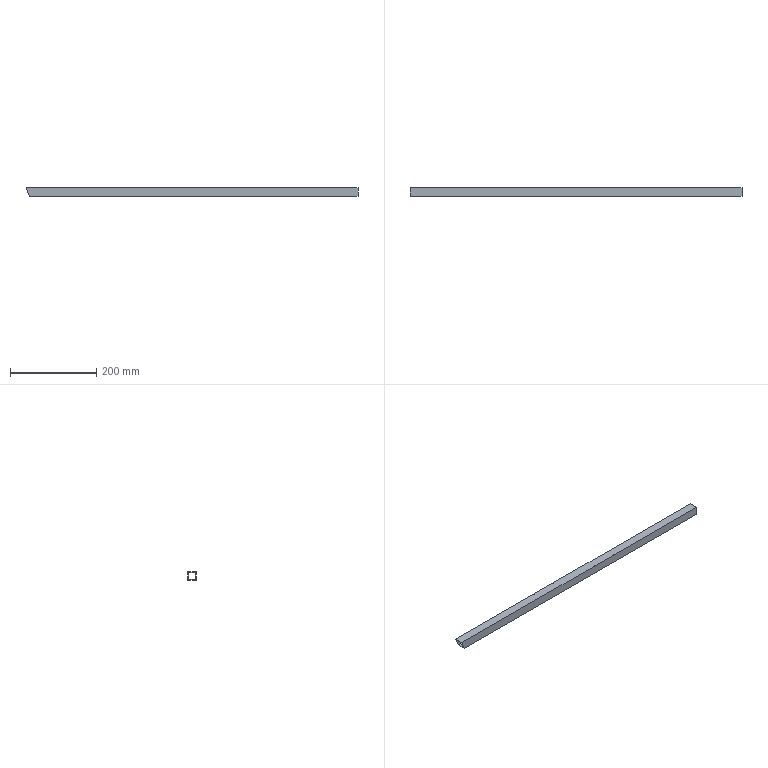Part | NX | features BREP 1 | 1 solid | 15 faces | box 768.614 x 20 x 20 mm | volume 110084 mm3 | plane 15
STEP:
#1=CARTESIAN_POINT('',(840.802,680.,1311.692));
#2=VERTEX_POINT('',#1);
#3=CARTESIAN_POINT('',(1608.587,680.,1311.692));
#4=VERTEX_POINT('',#3);
#5=CARTESIAN_POINT('',(1224.695,680.,1311.692));
#6=DIRECTION('',(1.,0.,0.));
#7=VECTOR('',#6,1000.);
#8=LINE('',#5,#7);
#9=EDGE_CURVE('',#2,#4,#8,.T.);
#10=ORIENTED_EDGE('',*,*,#9,.T.);
#11=CARTESIAN_POINT('',(1608.587,680.,1295.692));
#12=VERTEX_POINT('',#11);
#13=CARTESIAN_POINT('',(1608.587,680.,1303.692));
#14=DIRECTION('',(0.,0.,1.));
#15=VECTOR('',#14,1000.);
#16=LINE('',#13,#15);
#17=EDGE_CURVE('',#12,#4,#16,.T.);
#18=ORIENTED_EDGE('',*,*,#17,.F.);
#19=CARTESIAN_POINT('',(847.429,680.,1295.692));
#20=VERTEX_POINT('',#19);
#21=CARTESIAN_POINT('',(1228.008,680.,1295.692));
#22=DIRECTION('',(1.,0.,0.));
#23=VECTOR('',#22,1000.);
#24=LINE('',#21,#23);
#25=EDGE_CURVE('',#20,#12,#24,.T.);
#26=ORIENTED_EDGE('',*,*,#25,.F.);
#27=CARTESIAN_POINT('',(844.116,680.,1303.692));
#28=DIRECTION('',(-0.3827,0.,0.9239));
#29=VECTOR('',#28,1000.);
#30=LINE('',#27,#29);
#31=EDGE_CURVE('',#20,#2,#30,.T.);
#32=ORIENTED_EDGE('',*,*,#31,.T.);
#33=EDGE_LOOP('',(#10,#18,#26,#32));
#34=FACE_BOUND('',#33,.T.);
#35=CARTESIAN_POINT('',(657.176,680.,1313.692));
#36=DIRECTION('',(0.,1.,0.));
#37=DIRECTION('',(1.,0.,0.));
#38=AXIS2_PLACEMENT_3D('',#35,#36,#37);
#39=PLANE('',#38);
#40=ADVANCED_FACE('',(#34),#39,.T.);
#41=CARTESIAN_POINT('',(839.974,678.,1313.692));
#42=VERTEX_POINT('',#41);
#43=CARTESIAN_POINT('',(848.258,678.,1293.692));
#44=VERTEX_POINT('',#43);
#45=CARTESIAN_POINT('',(844.116,678.,1303.692));
#46=DIRECTION('',(0.3827,0.,-0.9239));
#47=VECTOR('',#46,1000.);
#48=LINE('',#45,#47);
#49=EDGE_CURVE('',#42,#44,#48,.T.);
#50=ORIENTED_EDGE('',*,*,#49,.T.);
#51=CARTESIAN_POINT('',(1608.587,678.,1293.692));
#52=VERTEX_POINT('',#51);
#53=CARTESIAN_POINT('',(1228.423,678.,1293.692));
#54=DIRECTION('',(1.,0.,0.));
#55=VECTOR('',#54,1000.);
#56=LINE('',#53,#55);
#57=EDGE_CURVE('',#44,#52,#56,.T.);
#58=ORIENTED_EDGE('',*,*,#57,.T.);
#59=CARTESIAN_POINT('',(1608.587,678.,1313.692));
#60=VERTEX_POINT('',#59);
#61=CARTESIAN_POINT('',(1608.587,678.,1303.692));
#62=DIRECTION('',(0.,0.,1.));
#63=VECTOR('',#62,1000.);
#64=LINE('',#61,#63);
#65=EDGE_CURVE('',#52,#60,#64,.T.);
#66=ORIENTED_EDGE('',*,*,#65,.T.);
#67=CARTESIAN_POINT('',(1224.28,678.,1313.692));
#68=DIRECTION('',(1.,0.,0.));
#69=VECTOR('',#68,1000.);
#70=LINE('',#67,#69);
#71=EDGE_CURVE('',#42,#60,#70,.T.);
#72=ORIENTED_EDGE('',*,*,#71,.F.);
#73=EDGE_LOOP('',(#50,#58,#66,#72));
#74=FACE_BOUND('',#73,.T.);
#75=CARTESIAN_POINT('',(657.176,678.,1313.692));
#76=DIRECTION('',(0.,1.,0.));
#77=DIRECTION('',(1.,0.,0.));
#78=AXIS2_PLACEMENT_3D('',#75,#76,#77);
#79=PLANE('',#78);
#80=ADVANCED_FACE('',(#74),#79,.F.);
#81=CARTESIAN_POINT('',(1608.587,680.,1293.692));
#82=VERTEX_POINT('',#81);
#83=CARTESIAN_POINT('',(1608.587,679.,1293.692));
#84=DIRECTION('',(0.,-1.,0.));
#85=VECTOR('',#84,1000.);
#86=LINE('',#83,#85);
#87=EDGE_CURVE('',#82,#52,#86,.T.);
#88=ORIENTED_EDGE('',*,*,#87,.F.);
#89=CARTESIAN_POINT('',(1608.587,680.,1294.692));
#90=DIRECTION('',(0.,0.,1.));
#91=VECTOR('',#90,1000.);
#92=LINE('',#89,#91);
#93=EDGE_CURVE('',#82,#12,#92,.T.);
#94=ORIENTED_EDGE('',*,*,#93,.T.);
#95=CARTESIAN_POINT('',(1608.587,679.,1294.692));
#96=DIRECTION('',(0.,0.7071,0.7071));
#97=VECTOR('',#96,1000.);
#98=LINE('',#95,#97);
#99=EDGE_CURVE('',#52,#12,#98,.T.);
#100=ORIENTED_EDGE('',*,*,#99,.F.);
#101=EDGE_LOOP('',(#88,#94,#100));
#102=FACE_BOUND('',#101,.T.);
#103=CARTESIAN_POINT('',(1608.587,678.,1303.692));
#104=DIRECTION('',(-1.,0.,0.));
#105=DIRECTION('',(0.,-1.,0.));
#106=AXIS2_PLACEMENT_3D('',#103,#104,#105);
#107=PLANE('',#106);
#108=ADVANCED_FACE('',(#102),#107,.F.);
#109=ORIENTED_EDGE('',*,*,#25,.T.);
#110=CARTESIAN_POINT('',(1608.587,696.,1295.692));
#111=VERTEX_POINT('',#110);
#112=CARTESIAN_POINT('',(1608.587,688.,1295.692));
#113=DIRECTION('',(0.,-1.,0.));
#114=VECTOR('',#113,1000.);
#115=LINE('',#112,#114);
#116=EDGE_CURVE('',#111,#12,#115,.T.);
#117=ORIENTED_EDGE('',*,*,#116,.F.);
#118=CARTESIAN_POINT('',(847.429,696.,1295.692));
#119=VERTEX_POINT('',#118);
#120=CARTESIAN_POINT('',(1228.008,696.,1295.692));
#121=DIRECTION('',(1.,0.,0.));
#122=VECTOR('',#121,1000.);
#123=LINE('',#120,#122);
#124=EDGE_CURVE('',#119,#111,#123,.T.);
#125=ORIENTED_EDGE('',*,*,#124,.F.);
#126=CARTESIAN_POINT('',(847.429,688.,1295.692));
#127=DIRECTION('',(0.,1.,0.));
#128=VECTOR('',#127,1000.);
#129=LINE('',#126,#128);
#130=EDGE_CURVE('',#20,#119,#129,.T.);
#131=ORIENTED_EDGE('',*,*,#130,.F.);
#132=EDGE_LOOP('',(#109,#117,#125,#131));
#133=FACE_BOUND('',#132,.T.);
#134=CARTESIAN_POINT('',(657.176,678.,1295.692));
#135=DIRECTION('',(0.,0.,1.));
#136=DIRECTION('',(1.,0.,0.));
#137=AXIS2_PLACEMENT_3D('',#134,#135,#136);
#138=PLANE('',#137);
#139=ADVANCED_FACE('',(#133),#138,.T.);
#140=CARTESIAN_POINT('',(840.802,696.,1311.692));
#141=VERTEX_POINT('',#140);
#142=CARTESIAN_POINT('',(1608.587,696.,1311.692));
#143=VERTEX_POINT('',#142);
#144=CARTESIAN_POINT('',(1224.695,696.,1311.692));
#145=DIRECTION('',(1.,0.,0.));
#146=VECTOR('',#145,1000.);
#147=LINE('',#144,#146);
#148=EDGE_CURVE('',#141,#143,#147,.T.);
#149=ORIENTED_EDGE('',*,*,#148,.T.);
#150=CARTESIAN_POINT('',(1608.587,688.,1311.692));
#151=DIRECTION('',(0.,-1.,0.));
#152=VECTOR('',#151,1000.);
#153=LINE('',#150,#152);
#154=EDGE_CURVE('',#143,#4,#153,.T.);
#155=ORIENTED_EDGE('',*,*,#154,.T.);
#156=ORIENTED_EDGE('',*,*,#9,.F.);
#157=CARTESIAN_POINT('',(840.802,688.,1311.692));
#158=DIRECTION('',(0.,-1.,0.));
#159=VECTOR('',#158,1000.);
#160=LINE('',#157,#159);
#161=EDGE_CURVE('',#141,#2,#160,.T.);
#162=ORIENTED_EDGE('',*,*,#161,.F.);
#163=EDGE_LOOP('',(#149,#155,#156,#162));
#164=FACE_BOUND('',#163,.T.);
#165=CARTESIAN_POINT('',(657.176,698.,1311.692));
#166=DIRECTION('',(0.,0.,-1.));
#167=DIRECTION('',(1.,0.,0.));
#168=AXIS2_PLACEMENT_3D('',#165,#166,#167);
#169=PLANE('',#168);
#170=ADVANCED_FACE('',(#164),#169,.T.);
#171=ORIENTED_EDGE('',*,*,#99,.T.);
#172=ORIENTED_EDGE('',*,*,#17,.T.);
#173=CARTESIAN_POINT('',(1608.587,679.,1312.692));
#174=DIRECTION('',(0.,0.7071,-0.7071));
#175=VECTOR('',#174,1000.);
#176=LINE('',#173,#175);
#177=EDGE_CURVE('',#60,#4,#176,.T.);
#178=ORIENTED_EDGE('',*,*,#177,.F.);
#179=ORIENTED_EDGE('',*,*,#65,.F.);
#180=EDGE_LOOP('',(#171,#172,#178,#179));
#181=FACE_BOUND('',#180,.T.);
#182=CARTESIAN_POINT('',(1608.587,678.,1303.692));
#183=DIRECTION('',(-1.,0.,0.));
#184=DIRECTION('',(0.,-1.,0.));
#185=AXIS2_PLACEMENT_3D('',#182,#183,#184);
#186=PLANE('',#185);
#187=ADVANCED_FACE('',(#181),#186,.F.);
#188=ORIENTED_EDGE('',*,*,#161,.T.);
#189=ORIENTED_EDGE('',*,*,#31,.F.);
#190=ORIENTED_EDGE('',*,*,#130,.T.);
#191=CARTESIAN_POINT('',(844.116,696.,1303.692));
#192=DIRECTION('',(0.3827,0.,-0.9239));
#193=VECTOR('',#192,1000.);
#194=LINE('',#191,#193);
#195=EDGE_CURVE('',#141,#119,#194,.T.);
#196=ORIENTED_EDGE('',*,*,#195,.F.);
#197=EDGE_LOOP('',(#188,#189,#190,#196));
#198=FACE_BOUND('',#197,.T.);
#199=CARTESIAN_POINT('',(839.974,698.,1313.692));
#200=VERTEX_POINT('',#199);
#201=CARTESIAN_POINT('',(848.258,698.,1293.692));
#202=VERTEX_POINT('',#201);
#203=CARTESIAN_POINT('',(839.974,698.,1313.692));
#204=CARTESIAN_POINT('',(848.258,698.,1293.692));
#205=B_SPLINE_CURVE_WITH_KNOTS('',1,(#203,#204),.UNSPECIFIED.,.F.,.F.,(2,2),(-10.824,10.824),.UNSPECIFIED.);
#206=EDGE_CURVE('',#200,#202,#205,.T.);
#207=ORIENTED_EDGE('',*,*,#206,.T.);
#208=CARTESIAN_POINT('',(848.258,688.,1293.692));
#209=DIRECTION('',(0.,-1.,0.));
#210=VECTOR('',#209,1000.);
#211=LINE('',#208,#210);
#212=EDGE_CURVE('',#202,#44,#211,.T.);
#213=ORIENTED_EDGE('',*,*,#212,.T.);
#214=ORIENTED_EDGE('',*,*,#49,.F.);
#215=CARTESIAN_POINT('',(839.974,688.,1313.692));
#216=DIRECTION('',(0.,-1.,0.));
#217=VECTOR('',#216,1000.);
#218=LINE('',#215,#217);
#219=EDGE_CURVE('',#200,#42,#218,.T.);
#220=ORIENTED_EDGE('',*,*,#219,.F.);
#221=EDGE_LOOP('',(#207,#213,#214,#220));
#222=FACE_BOUND('',#221,.T.);
#223=CARTESIAN_POINT('',(839.974,678.,1313.692));
#224=DIRECTION('',(0.9239,0.,0.3827));
#225=DIRECTION('',(0.3827,0.,-0.9239));
#226=AXIS2_PLACEMENT_3D('',#223,#224,#225);
#227=PLANE('',#226);
#228=ADVANCED_FACE('',(#198,#222),#227,.F.);
#229=ORIENTED_EDGE('',*,*,#219,.T.);
#230=ORIENTED_EDGE('',*,*,#71,.T.);
#231=CARTESIAN_POINT('',(1608.587,698.,1313.692));
#232=VERTEX_POINT('',#231);
#233=CARTESIAN_POINT('',(1608.587,688.,1313.692));
#234=DIRECTION('',(0.,-1.,0.));
#235=VECTOR('',#234,1000.);
#236=LINE('',#233,#235);
#237=EDGE_CURVE('',#232,#60,#236,.T.);
#238=ORIENTED_EDGE('',*,*,#237,.F.);
#239=CARTESIAN_POINT('',(839.974,698.,1313.692));
#240=CARTESIAN_POINT('',(993.696,698.,1313.692));
#241=CARTESIAN_POINT('',(1147.419,698.,1313.692));
#242=CARTESIAN_POINT('',(1301.142,698.,1313.692));
#243=CARTESIAN_POINT('',(1454.865,698.,1313.692));
#244=CARTESIAN_POINT('',(1608.587,698.,1313.692));
#245=B_SPLINE_CURVE_WITH_KNOTS('',5,(#239,#240,#241,#242,#243,#244),.UNSPECIFIED.,.F.,.F.,(6,6),(182.798,951.412),.UNSPECIFIED.);
#246=EDGE_CURVE('',#200,#232,#245,.T.);
#247=ORIENTED_EDGE('',*,*,#246,.F.);
#248=EDGE_LOOP('',(#229,#230,#238,#247));
#249=FACE_BOUND('',#248,.T.);
#250=CARTESIAN_POINT('',(657.176,698.,1313.692));
#251=DIRECTION('',(0.,0.,-1.));
#252=DIRECTION('',(1.,0.,0.));
#253=AXIS2_PLACEMENT_3D('',#250,#251,#252);
#254=PLANE('',#253);
#255=ADVANCED_FACE('',(#249),#254,.F.);
#256=ORIENTED_EDGE('',*,*,#212,.F.);
#257=CARTESIAN_POINT('',(1608.587,698.,1293.692));
#258=VERTEX_POINT('',#257);
#259=CARTESIAN_POINT('',(848.258,698.,1293.692));
#260=CARTESIAN_POINT('',(1000.324,698.,1293.692));
#261=CARTESIAN_POINT('',(1152.39,698.,1293.692));
#262=CARTESIAN_POINT('',(1304.456,698.,1293.692));
#263=CARTESIAN_POINT('',(1456.521,698.,1293.692));
#264=CARTESIAN_POINT('',(1608.587,698.,1293.692));
#265=B_SPLINE_CURVE_WITH_KNOTS('',5,(#259,#260,#261,#262,#263,#264),.UNSPECIFIED.,.F.,.F.,(6,6),(191.082,951.412),.UNSPECIFIED.);
#266=EDGE_CURVE('',#202,#258,#265,.T.);
#267=ORIENTED_EDGE('',*,*,#266,.T.);
#268=CARTESIAN_POINT('',(1608.587,696.,1293.692));
#269=VERTEX_POINT('',#268);
#270=CARTESIAN_POINT('',(1608.587,697.,1293.692));
#271=DIRECTION('',(0.,-1.,0.));
#272=VECTOR('',#271,1000.);
#273=LINE('',#270,#272);
#274=EDGE_CURVE('',#258,#269,#273,.T.);
#275=ORIENTED_EDGE('',*,*,#274,.T.);
#276=CARTESIAN_POINT('',(1608.587,688.,1293.692));
#277=DIRECTION('',(0.,-1.,0.));
#278=VECTOR('',#277,1000.);
#279=LINE('',#276,#278);
#280=EDGE_CURVE('',#269,#82,#279,.T.);
#281=ORIENTED_EDGE('',*,*,#280,.T.);
#282=ORIENTED_EDGE('',*,*,#87,.T.);
#283=ORIENTED_EDGE('',*,*,#57,.F.);
#284=EDGE_LOOP('',(#256,#267,#275,#281,#282,#283));
#285=FACE_BOUND('',#284,.T.);
#286=CARTESIAN_POINT('',(657.176,678.,1293.692));
#287=DIRECTION('',(0.,0.,1.));
#288=DIRECTION('',(1.,0.,0.));
#289=AXIS2_PLACEMENT_3D('',#286,#287,#288);
#290=PLANE('',#289);
#291=ADVANCED_FACE('',(#285),#290,.F.);
#292=CARTESIAN_POINT('',(1608.587,696.,1294.692));
#293=DIRECTION('',(0.,0.,1.));
#294=VECTOR('',#293,1000.);
#295=LINE('',#292,#294);
#296=EDGE_CURVE('',#269,#111,#295,.T.);
#297=ORIENTED_EDGE('',*,*,#296,.T.);
#298=ORIENTED_EDGE('',*,*,#116,.T.);
#299=ORIENTED_EDGE('',*,*,#93,.F.);
#300=ORIENTED_EDGE('',*,*,#280,.F.);
#301=EDGE_LOOP('',(#297,#298,#299,#300));
#302=FACE_BOUND('',#301,.T.);
#303=CARTESIAN_POINT('',(1608.587,689.,1293.692));
#304=DIRECTION('',(-1.,0.,0.));
#305=DIRECTION('',(0.,-1.,0.));
#306=AXIS2_PLACEMENT_3D('',#303,#304,#305);
#307=PLANE('',#306);
#308=ADVANCED_FACE('',(#302),#307,.F.);
#309=ORIENTED_EDGE('',*,*,#195,.T.);
#310=ORIENTED_EDGE('',*,*,#124,.T.);
#311=CARTESIAN_POINT('',(1608.587,696.,1303.692));
#312=DIRECTION('',(0.,0.,-1.));
#313=VECTOR('',#312,1000.);
#314=LINE('',#311,#313);
#315=EDGE_CURVE('',#143,#111,#314,.T.);
#316=ORIENTED_EDGE('',*,*,#315,.F.);
#317=ORIENTED_EDGE('',*,*,#148,.F.);
#318=EDGE_LOOP('',(#309,#310,#316,#317));
#319=FACE_BOUND('',#318,.T.);
#320=CARTESIAN_POINT('',(840.802,696.,1311.692));
#321=DIRECTION('',(0.,1.,0.));
#322=DIRECTION('',(1.,0.,0.));
#323=AXIS2_PLACEMENT_3D('',#320,#321,#322);
#324=PLANE('',#323);
#325=ADVANCED_FACE('',(#319),#324,.F.);
#326=ORIENTED_EDGE('',*,*,#177,.T.);
#327=ORIENTED_EDGE('',*,*,#154,.F.);
#328=CARTESIAN_POINT('',(1608.587,697.,1312.692));
#329=DIRECTION('',(0.,-0.7071,-0.7071));
#330=VECTOR('',#329,1000.);
#331=LINE('',#328,#330);
#332=EDGE_CURVE('',#232,#143,#331,.T.);
#333=ORIENTED_EDGE('',*,*,#332,.F.);
#334=ORIENTED_EDGE('',*,*,#237,.T.);
#335=EDGE_LOOP('',(#326,#327,#333,#334));
#336=FACE_BOUND('',#335,.T.);
#337=CARTESIAN_POINT('',(1608.587,688.,1313.692));
#338=DIRECTION('',(1.,0.,0.));
#339=DIRECTION('',(0.,-1.,0.));
#340=AXIS2_PLACEMENT_3D('',#337,#338,#339);
#341=PLANE('',#340);
#342=ADVANCED_FACE('',(#336),#341,.T.);
#343=ORIENTED_EDGE('',*,*,#246,.T.);
#344=CARTESIAN_POINT('',(1608.587,698.,1303.692));
#345=DIRECTION('',(0.,0.,-1.));
#346=VECTOR('',#345,1000.);
#347=LINE('',#344,#346);
#348=EDGE_CURVE('',#232,#258,#347,.T.);
#349=ORIENTED_EDGE('',*,*,#348,.T.);
#350=ORIENTED_EDGE('',*,*,#266,.F.);
#351=ORIENTED_EDGE('',*,*,#206,.F.);
#352=EDGE_LOOP('',(#343,#349,#350,#351));
#353=FACE_BOUND('',#352,.T.);
#354=CARTESIAN_POINT('',(1253.676,698.,1303.692));
#355=DIRECTION('',(0.,1.,0.));
#356=DIRECTION('',(0.,0.,1.));
#357=AXIS2_PLACEMENT_3D('',#354,#355,#356);
#358=PLANE('',#357);
#359=ADVANCED_FACE('',(#353),#358,.T.);
#360=ORIENTED_EDGE('',*,*,#296,.F.);
#361=ORIENTED_EDGE('',*,*,#274,.F.);
#362=CARTESIAN_POINT('',(1608.587,697.,1294.692));
#363=DIRECTION('',(0.,-0.7071,0.7071));
#364=VECTOR('',#363,1000.);
#365=LINE('',#362,#364);
#366=EDGE_CURVE('',#258,#111,#365,.T.);
#367=ORIENTED_EDGE('',*,*,#366,.T.);
#368=EDGE_LOOP('',(#360,#361,#367));
#369=FACE_BOUND('',#368,.T.);
#370=CARTESIAN_POINT('',(1608.587,698.,1313.692));
#371=DIRECTION('',(-1.,0.,0.));
#372=DIRECTION('',(0.,0.,-1.));
#373=AXIS2_PLACEMENT_3D('',#370,#371,#372);
#374=PLANE('',#373);
#375=ADVANCED_FACE('',(#369),#374,.F.);
#376=ORIENTED_EDGE('',*,*,#366,.F.);
#377=ORIENTED_EDGE('',*,*,#348,.F.);
#378=ORIENTED_EDGE('',*,*,#332,.T.);
#379=ORIENTED_EDGE('',*,*,#315,.T.);
#380=EDGE_LOOP('',(#376,#377,#378,#379));
#381=FACE_BOUND('',#380,.T.);
#382=CARTESIAN_POINT('',(1608.587,698.,1313.692));
#383=DIRECTION('',(-1.,0.,0.));
#384=DIRECTION('',(0.,0.,-1.));
#385=AXIS2_PLACEMENT_3D('',#382,#383,#384);
#386=PLANE('',#385);
#387=ADVANCED_FACE('',(#381),#386,.F.);
#388=CLOSED_SHELL('',(#40,#80,#108,#139,#170,#187,#228,#255,#291,#308,#325,#342,#359,#375,#387));
#389=MANIFOLD_SOLID_BREP('',#388);
#390=(LENGTH_UNIT()NAMED_UNIT(*)SI_UNIT(.MILLI.,.METRE.));
#391=UNCERTAINTY_MEASURE_WITH_UNIT(LENGTH_MEASURE(0.00001),#390,'','');
#392=(NAMED_UNIT(*)PLANE_ANGLE_UNIT()SI_UNIT($,.RADIAN.));
#393=(NAMED_UNIT(*)SI_UNIT($,.STERADIAN.)SOLID_ANGLE_UNIT());
#394=(GEOMETRIC_REPRESENTATION_CONTEXT(3)GLOBAL_UNCERTAINTY_ASSIGNED_CONTEXT((#391))GLOBAL_UNIT_ASSIGNED_CONTEXT((#390,#392,#393))REPRESENTATION_CONTEXT('',''));
#395=ADVANCED_BREP_SHAPE_REPRESENTATION('',(#389),#394);